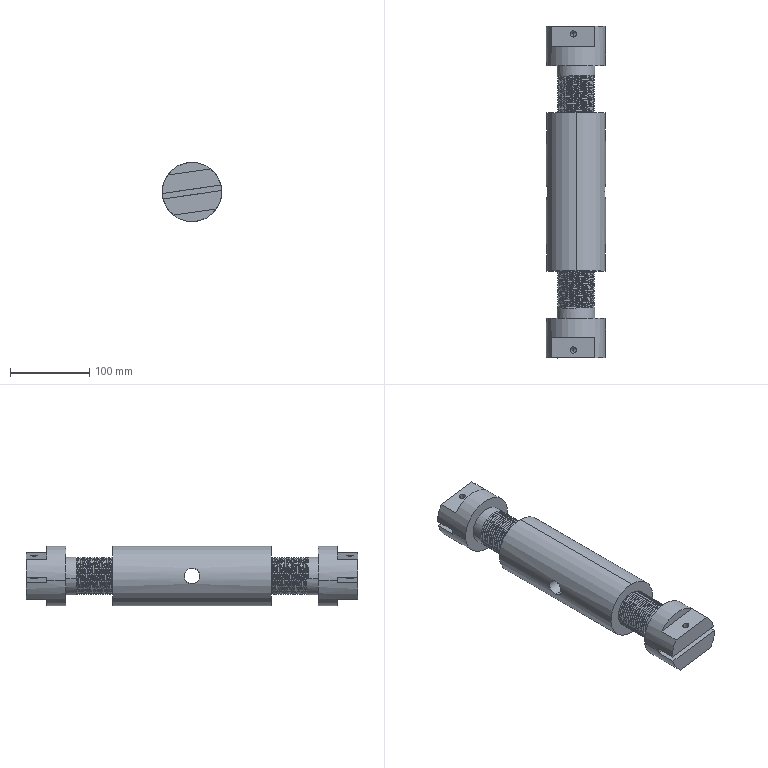Part | SolidWorks | 3 solids | 380 faces | box 75 x 420 x 75 mm | volume 1306901 mm3 | cylinder 298 | spline 48 | plane 30 | cone 4 | commonest cylinder face diameters 48 x280 8 x8 75 x6 20 x4